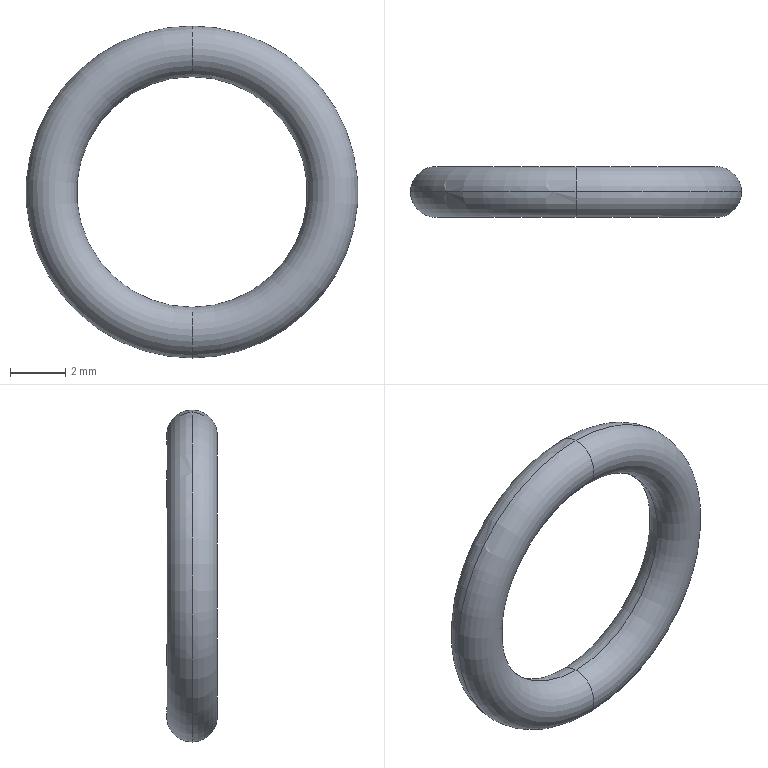Part | SolidWorks | features Sweep 1 | 1 solid | 4 faces | box 12.043 x 1.84 x 12.043 mm | volume 85.235 mm3 | torus 4
STEP:
#1=CARTESIAN_POINT('',(0.,0.,-6.022));
#2=VERTEX_POINT('',#1);
#3=CARTESIAN_POINT('',(0.,0.,-4.182));
#4=VERTEX_POINT('',#3);
#5=CARTESIAN_POINT('',(0.,0.,-5.102));
#6=DIRECTION('',(1.,0.,0.));
#7=DIRECTION('',(0.,0.,-1.));
#8=AXIS2_PLACEMENT_3D('',#5,#6,#7);
#9=CIRCLE('',#8,0.92);
#10=EDGE_CURVE('',#2,#4,#9,.T.);
#11=ORIENTED_EDGE('',*,*,#10,.F.);
#12=CARTESIAN_POINT('',(0.,0.,6.022));
#13=VERTEX_POINT('',#12);
#14=CARTESIAN_POINT('',(0.,0.,0.));
#15=DIRECTION('',(0.,1.,0.));
#16=DIRECTION('',(0.,0.,1.));
#17=AXIS2_PLACEMENT_3D('',#14,#15,#16);
#18=CIRCLE('',#17,6.022);
#19=EDGE_CURVE('',#2,#13,#18,.T.);
#20=ORIENTED_EDGE('',*,*,#19,.T.);
#21=CARTESIAN_POINT('',(0.,0.,4.182));
#22=VERTEX_POINT('',#21);
#23=CARTESIAN_POINT('',(0.,0.,5.102));
#24=DIRECTION('',(-1.,0.,0.));
#25=DIRECTION('',(0.,0.,1.));
#26=AXIS2_PLACEMENT_3D('',#23,#24,#25);
#27=CIRCLE('',#26,0.92);
#28=EDGE_CURVE('',#13,#22,#27,.T.);
#29=ORIENTED_EDGE('',*,*,#28,.T.);
#30=CARTESIAN_POINT('',(0.,0.,0.));
#31=DIRECTION('',(0.,1.,0.));
#32=DIRECTION('',(0.,0.,1.));
#33=AXIS2_PLACEMENT_3D('',#30,#31,#32);
#34=CIRCLE('',#33,4.182);
#35=EDGE_CURVE('',#4,#22,#34,.T.);
#36=ORIENTED_EDGE('',*,*,#35,.F.);
#37=EDGE_LOOP('',(#11,#20,#29,#36));
#38=FACE_OUTER_BOUND('',#37,.T.);
#39=CARTESIAN_POINT('',(0.,0.,0.));
#40=DIRECTION('',(0.,1.,0.));
#41=DIRECTION('',(0.,0.,1.));
#42=AXIS2_PLACEMENT_3D('',#39,#40,#41);
#43=TOROIDAL_SURFACE('',#42,5.102,0.92);
#44=ADVANCED_FACE('',(#38),#43,.T.);
#45=ORIENTED_EDGE('',*,*,#28,.F.);
#46=CARTESIAN_POINT('',(0.,0.,0.));
#47=DIRECTION('',(0.,1.,0.));
#48=DIRECTION('',(0.,0.,1.));
#49=AXIS2_PLACEMENT_3D('',#46,#47,#48);
#50=CIRCLE('',#49,6.022);
#51=EDGE_CURVE('',#13,#2,#50,.T.);
#52=ORIENTED_EDGE('',*,*,#51,.T.);
#53=ORIENTED_EDGE('',*,*,#10,.T.);
#54=CARTESIAN_POINT('',(0.,0.,0.));
#55=DIRECTION('',(0.,1.,0.));
#56=DIRECTION('',(0.,0.,1.));
#57=AXIS2_PLACEMENT_3D('',#54,#55,#56);
#58=CIRCLE('',#57,4.182);
#59=EDGE_CURVE('',#22,#4,#58,.T.);
#60=ORIENTED_EDGE('',*,*,#59,.F.);
#61=EDGE_LOOP('',(#45,#52,#53,#60));
#62=FACE_OUTER_BOUND('',#61,.T.);
#63=CARTESIAN_POINT('',(0.,0.,0.));
#64=DIRECTION('',(0.,1.,0.));
#65=DIRECTION('',(0.,0.,1.));
#66=AXIS2_PLACEMENT_3D('',#63,#64,#65);
#67=TOROIDAL_SURFACE('',#66,5.102,0.92);
#68=ADVANCED_FACE('',(#62),#67,.T.);
#69=ORIENTED_EDGE('',*,*,#51,.F.);
#70=CARTESIAN_POINT('',(0.,0.,5.102));
#71=DIRECTION('',(-1.,0.,0.));
#72=DIRECTION('',(0.,0.,1.));
#73=AXIS2_PLACEMENT_3D('',#70,#71,#72);
#74=CIRCLE('',#73,0.92);
#75=EDGE_CURVE('',#22,#13,#74,.T.);
#76=ORIENTED_EDGE('',*,*,#75,.F.);
#77=ORIENTED_EDGE('',*,*,#59,.T.);
#78=CARTESIAN_POINT('',(0.,0.,-5.102));
#79=DIRECTION('',(1.,0.,0.));
#80=DIRECTION('',(0.,0.,-1.));
#81=AXIS2_PLACEMENT_3D('',#78,#79,#80);
#82=CIRCLE('',#81,0.92);
#83=EDGE_CURVE('',#4,#2,#82,.T.);
#84=ORIENTED_EDGE('',*,*,#83,.T.);
#85=EDGE_LOOP('',(#69,#76,#77,#84));
#86=FACE_OUTER_BOUND('',#85,.T.);
#87=CARTESIAN_POINT('',(0.,0.,0.));
#88=DIRECTION('',(0.,1.,0.));
#89=DIRECTION('',(0.,0.,1.));
#90=AXIS2_PLACEMENT_3D('',#87,#88,#89);
#91=TOROIDAL_SURFACE('',#90,5.102,0.92);
#92=ADVANCED_FACE('',(#86),#91,.T.);
#93=ORIENTED_EDGE('',*,*,#19,.F.);
#94=ORIENTED_EDGE('',*,*,#83,.F.);
#95=ORIENTED_EDGE('',*,*,#35,.T.);
#96=ORIENTED_EDGE('',*,*,#75,.T.);
#97=EDGE_LOOP('',(#93,#94,#95,#96));
#98=FACE_OUTER_BOUND('',#97,.T.);
#99=CARTESIAN_POINT('',(0.,0.,0.));
#100=DIRECTION('',(0.,1.,0.));
#101=DIRECTION('',(0.,0.,1.));
#102=AXIS2_PLACEMENT_3D('',#99,#100,#101);
#103=TOROIDAL_SURFACE('',#102,5.102,0.92);
#104=ADVANCED_FACE('',(#98),#103,.T.);
#105=CLOSED_SHELL('',(#44,#68,#92,#104));
#106=MANIFOLD_SOLID_BREP('',#105);
#107=CARTESIAN_POINT('',(0.,0.,0.));
#108=DIRECTION('',(0.,0.,1.));
#109=DIRECTION('',(1.,0.,0.));
#110=AXIS2_PLACEMENT_3D('',#107,#108,#109);
#111=(LENGTH_UNIT()NAMED_UNIT(*)SI_UNIT(.MILLI.,.METRE.));
#112=UNCERTAINTY_MEASURE_WITH_UNIT(LENGTH_MEASURE(0.00001),#111,'','');
#113=(NAMED_UNIT(*)PLANE_ANGLE_UNIT()SI_UNIT($,.RADIAN.));
#114=(NAMED_UNIT(*)SI_UNIT($,.STERADIAN.)SOLID_ANGLE_UNIT());
#115=(GEOMETRIC_REPRESENTATION_CONTEXT(3)GLOBAL_UNCERTAINTY_ASSIGNED_CONTEXT((#112))GLOBAL_UNIT_ASSIGNED_CONTEXT((#111,#113,#114))REPRESENTATION_CONTEXT('',''));
#116=ADVANCED_BREP_SHAPE_REPRESENTATION('',(#106,#110),#115);